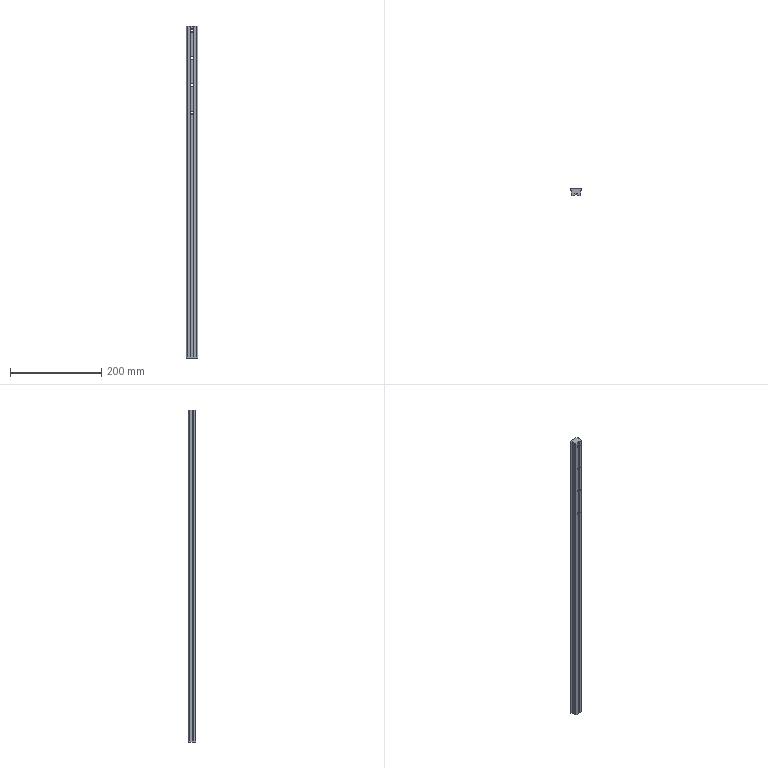Part | SolidWorks | features BaseBody 1 | 1 solid | 58 faces | box 25 x 16 x 728 mm | volume 224538 mm3 | plane 42 | cylinder 16 | commonest cylinder face diameters 7 x8 11 x8